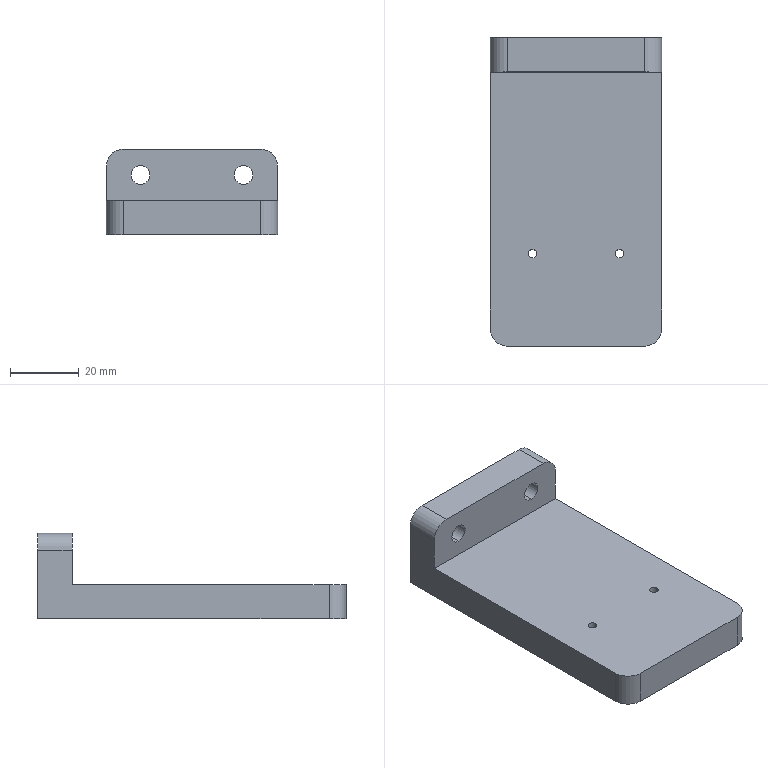Part | STEP file | PN_0021 | 1 solid | 20 faces | box 50 x 90 x 25 mm | volume 51712 mm3 | cylinder 12 | plane 8 | commonest cylinder face diameters 2.5 x4 5.5 x4 10 x4